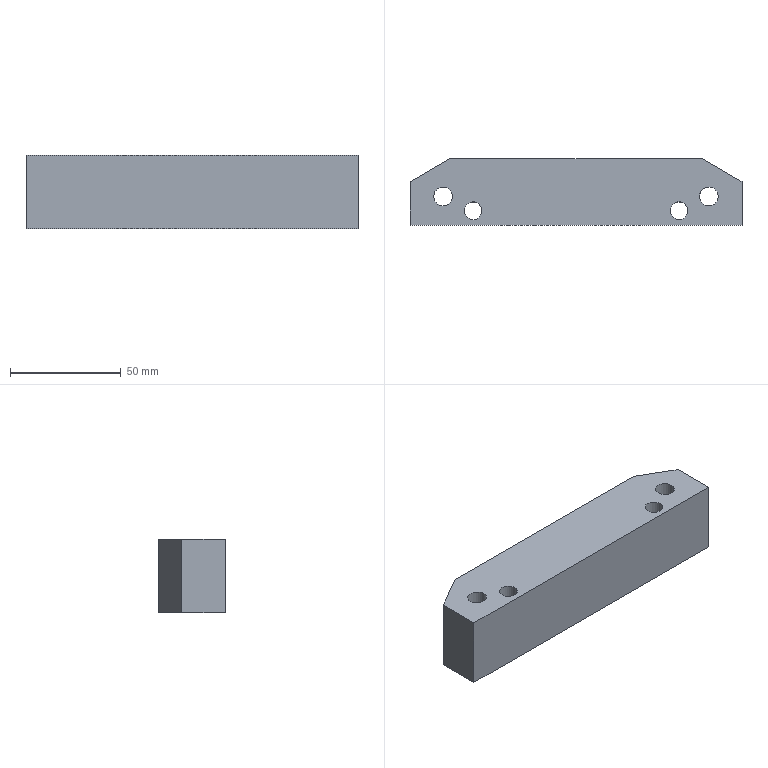Part | CATIA | 1 solid | 16 faces | box 150 x 30 x 33 mm | volume 135264 mm3 | plane 8 | cylinder 8 | commonest cylinder face diameters 8 x4 8.5 x4
STEP:
#1=CARTESIAN_POINT('',(75.,-30.,38.));
#2=VERTEX_POINT('',#1);
#3=CARTESIAN_POINT('',(75.,-30.,5.));
#4=VERTEX_POINT('',#3);
#5=CARTESIAN_POINT('',(75.,-30.,21.5));
#6=DIRECTION('',(0.,0.,-1.));
#7=VECTOR('',#6,1.);
#8=LINE('',#5,#7);
#9=EDGE_CURVE('',#2,#4,#8,.T.);
#10=ORIENTED_EDGE('',*,*,#9,.F.);
#11=CARTESIAN_POINT('',(-75.,-30.,38.));
#12=VERTEX_POINT('',#11);
#13=CARTESIAN_POINT('',(0.,-30.,38.));
#14=DIRECTION('',(-1.,0.,0.));
#15=VECTOR('',#14,1.);
#16=LINE('',#13,#15);
#17=EDGE_CURVE('',#2,#12,#16,.T.);
#18=ORIENTED_EDGE('',*,*,#17,.T.);
#19=CARTESIAN_POINT('',(-75.,-30.,5.));
#20=VERTEX_POINT('',#19);
#21=CARTESIAN_POINT('',(-75.,-30.,21.5));
#22=DIRECTION('',(0.,0.,-1.));
#23=VECTOR('',#22,1.);
#24=LINE('',#21,#23);
#25=EDGE_CURVE('',#12,#20,#24,.T.);
#26=ORIENTED_EDGE('',*,*,#25,.T.);
#27=CARTESIAN_POINT('',(0.,-30.,5.));
#28=DIRECTION('',(-1.,0.,0.));
#29=VECTOR('',#28,1.);
#30=LINE('',#27,#29);
#31=EDGE_CURVE('',#4,#20,#30,.T.);
#32=ORIENTED_EDGE('',*,*,#31,.F.);
#33=EDGE_LOOP('',(#10,#18,#26,#32));
#34=FACE_OUTER_BOUND('',#33,.T.);
#35=CARTESIAN_POINT('',(75.,-30.,38.));
#36=DIRECTION('',(0.,-1.,0.));
#37=DIRECTION('',(-1.,0.,0.));
#38=AXIS2_PLACEMENT_3D('',#35,#36,#37);
#39=PLANE('',#38);
#40=ADVANCED_FACE('',(#34),#39,.T.);
#41=CARTESIAN_POINT('',(-75.,-10.392,38.));
#42=VERTEX_POINT('',#41);
#43=CARTESIAN_POINT('',(-75.,-10.392,5.));
#44=VERTEX_POINT('',#43);
#45=CARTESIAN_POINT('',(-75.,-10.392,21.5));
#46=DIRECTION('',(0.,0.,-1.));
#47=VECTOR('',#46,1.);
#48=LINE('',#45,#47);
#49=EDGE_CURVE('',#42,#44,#48,.T.);
#50=ORIENTED_EDGE('',*,*,#49,.T.);
#51=CARTESIAN_POINT('',(-75.,-20.196,5.));
#52=DIRECTION('',(0.,-1.,0.));
#53=VECTOR('',#52,1.);
#54=LINE('',#51,#53);
#55=EDGE_CURVE('',#20,#44,#54,.F.);
#56=ORIENTED_EDGE('',*,*,#55,.F.);
#57=ORIENTED_EDGE('',*,*,#25,.F.);
#58=CARTESIAN_POINT('',(-75.,-20.196,38.));
#59=DIRECTION('',(0.,-1.,0.));
#60=VECTOR('',#59,1.);
#61=LINE('',#58,#60);
#62=EDGE_CURVE('',#12,#42,#61,.F.);
#63=ORIENTED_EDGE('',*,*,#62,.T.);
#64=EDGE_LOOP('',(#50,#56,#57,#63));
#65=FACE_OUTER_BOUND('',#64,.T.);
#66=CARTESIAN_POINT('',(-75.,0.,38.));
#67=DIRECTION('',(1.,0.,0.));
#68=DIRECTION('',(0.,-1.,0.));
#69=AXIS2_PLACEMENT_3D('',#66,#67,#68);
#70=PLANE('',#69);
#71=ADVANCED_FACE('',(#65),#70,.F.);
#72=CARTESIAN_POINT('',(-57.,0.,5.));
#73=VERTEX_POINT('',#72);
#74=CARTESIAN_POINT('',(-66.,-5.196,5.));
#75=DIRECTION('',(-0.866,-0.5,0.));
#76=VECTOR('',#75,1.);
#77=LINE('',#74,#76);
#78=EDGE_CURVE('',#73,#44,#77,.T.);
#79=ORIENTED_EDGE('',*,*,#78,.T.);
#80=ORIENTED_EDGE('',*,*,#49,.F.);
#81=CARTESIAN_POINT('',(-57.,0.,38.));
#82=VERTEX_POINT('',#81);
#83=CARTESIAN_POINT('',(-66.,-5.196,38.));
#84=DIRECTION('',(-0.866,-0.5,0.));
#85=VECTOR('',#84,1.);
#86=LINE('',#83,#85);
#87=EDGE_CURVE('',#42,#82,#86,.F.);
#88=ORIENTED_EDGE('',*,*,#87,.T.);
#89=CARTESIAN_POINT('',(-57.,0.,21.5));
#90=DIRECTION('',(0.,0.,-1.));
#91=VECTOR('',#90,1.);
#92=LINE('',#89,#91);
#93=EDGE_CURVE('',#82,#73,#92,.T.);
#94=ORIENTED_EDGE('',*,*,#93,.T.);
#95=EDGE_LOOP('',(#79,#80,#88,#94));
#96=FACE_OUTER_BOUND('',#95,.T.);
#97=CARTESIAN_POINT('',(-57.,0.,44.6));
#98=DIRECTION('',(-0.5,0.866,0.));
#99=DIRECTION('',(0.,0.,-1.));
#100=AXIS2_PLACEMENT_3D('',#97,#98,#99);
#101=PLANE('',#100);
#102=ADVANCED_FACE('',(#96),#101,.T.);
#103=CARTESIAN_POINT('',(75.,-10.392,38.));
#104=VERTEX_POINT('',#103);
#105=CARTESIAN_POINT('',(75.,-10.392,5.));
#106=VERTEX_POINT('',#105);
#107=CARTESIAN_POINT('',(75.,-10.392,21.5));
#108=DIRECTION('',(0.,0.,1.));
#109=VECTOR('',#108,1.);
#110=LINE('',#107,#109);
#111=EDGE_CURVE('',#104,#106,#110,.F.);
#112=ORIENTED_EDGE('',*,*,#111,.F.);
#113=CARTESIAN_POINT('',(75.,-20.196,38.));
#114=DIRECTION('',(0.,1.,0.));
#115=VECTOR('',#114,1.);
#116=LINE('',#113,#115);
#117=EDGE_CURVE('',#104,#2,#116,.F.);
#118=ORIENTED_EDGE('',*,*,#117,.T.);
#119=ORIENTED_EDGE('',*,*,#9,.T.);
#120=CARTESIAN_POINT('',(75.,-20.196,5.));
#121=DIRECTION('',(0.,1.,0.));
#122=VECTOR('',#121,1.);
#123=LINE('',#120,#122);
#124=EDGE_CURVE('',#106,#4,#123,.F.);
#125=ORIENTED_EDGE('',*,*,#124,.F.);
#126=EDGE_LOOP('',(#112,#118,#119,#125));
#127=FACE_OUTER_BOUND('',#126,.T.);
#128=CARTESIAN_POINT('',(75.,-30.,38.));
#129=DIRECTION('',(-1.,0.,0.));
#130=DIRECTION('',(0.,1.,0.));
#131=AXIS2_PLACEMENT_3D('',#128,#129,#130);
#132=PLANE('',#131);
#133=ADVANCED_FACE('',(#127),#132,.F.);
#134=CARTESIAN_POINT('',(57.,0.,5.));
#135=VERTEX_POINT('',#134);
#136=CARTESIAN_POINT('',(0.,0.,5.));
#137=DIRECTION('',(1.,0.,0.));
#138=VECTOR('',#137,1.);
#139=LINE('',#136,#138);
#140=EDGE_CURVE('',#73,#135,#139,.T.);
#141=ORIENTED_EDGE('',*,*,#140,.F.);
#142=ORIENTED_EDGE('',*,*,#93,.F.);
#143=CARTESIAN_POINT('',(57.,0.,38.));
#144=VERTEX_POINT('',#143);
#145=CARTESIAN_POINT('',(0.,0.,38.));
#146=DIRECTION('',(1.,0.,0.));
#147=VECTOR('',#146,1.);
#148=LINE('',#145,#147);
#149=EDGE_CURVE('',#82,#144,#148,.T.);
#150=ORIENTED_EDGE('',*,*,#149,.T.);
#151=CARTESIAN_POINT('',(57.,0.,21.5));
#152=DIRECTION('',(0.,0.,1.));
#153=VECTOR('',#152,1.);
#154=LINE('',#151,#153);
#155=EDGE_CURVE('',#144,#135,#154,.F.);
#156=ORIENTED_EDGE('',*,*,#155,.T.);
#157=EDGE_LOOP('',(#141,#142,#150,#156));
#158=FACE_OUTER_BOUND('',#157,.T.);
#159=CARTESIAN_POINT('',(-75.,0.,38.));
#160=DIRECTION('',(0.,1.,0.));
#161=DIRECTION('',(1.,0.,0.));
#162=AXIS2_PLACEMENT_3D('',#159,#160,#161);
#163=PLANE('',#162);
#164=ADVANCED_FACE('',(#158),#163,.T.);
#165=CARTESIAN_POINT('',(66.,-5.196,5.));
#166=DIRECTION('',(0.866,-0.5,0.));
#167=VECTOR('',#166,1.);
#168=LINE('',#165,#167);
#169=EDGE_CURVE('',#106,#135,#168,.F.);
#170=ORIENTED_EDGE('',*,*,#169,.T.);
#171=ORIENTED_EDGE('',*,*,#155,.F.);
#172=CARTESIAN_POINT('',(66.,-5.196,38.));
#173=DIRECTION('',(0.866,-0.5,0.));
#174=VECTOR('',#173,1.);
#175=LINE('',#172,#174);
#176=EDGE_CURVE('',#144,#104,#175,.T.);
#177=ORIENTED_EDGE('',*,*,#176,.T.);
#178=ORIENTED_EDGE('',*,*,#111,.T.);
#179=EDGE_LOOP('',(#170,#171,#177,#178));
#180=FACE_OUTER_BOUND('',#179,.T.);
#181=CARTESIAN_POINT('',(57.,0.,-1.6));
#182=DIRECTION('',(0.5,0.866,0.));
#183=DIRECTION('',(0.,0.,1.));
#184=AXIS2_PLACEMENT_3D('',#181,#182,#183);
#185=PLANE('',#184);
#186=ADVANCED_FACE('',(#180),#185,.T.);
#187=ORIENTED_EDGE('',*,*,#124,.T.);
#188=ORIENTED_EDGE('',*,*,#31,.T.);
#189=ORIENTED_EDGE('',*,*,#55,.T.);
#190=ORIENTED_EDGE('',*,*,#78,.F.);
#191=ORIENTED_EDGE('',*,*,#140,.T.);
#192=ORIENTED_EDGE('',*,*,#169,.F.);
#193=EDGE_LOOP('',(#187,#188,#189,#190,#191,#192));
#194=FACE_OUTER_BOUND('',#193,.T.);
#195=CARTESIAN_POINT('',(-63.73,-14.962,5.));
#196=VERTEX_POINT('',#195);
#197=CARTESIAN_POINT('',(-56.27,-19.038,5.));
#198=VERTEX_POINT('',#197);
#199=CARTESIAN_POINT('',(-60.,-17.,5.));
#200=DIRECTION('',(0.,0.,-1.));
#201=AXIS2_PLACEMENT_3D('',#199,#200,$);
#202=CIRCLE('',#201,4.25);
#203=EDGE_CURVE('',#196,#198,#202,.T.);
#204=ORIENTED_EDGE('',*,*,#203,.F.);
#205=CARTESIAN_POINT('',(-60.,-17.,5.));
#206=DIRECTION('',(0.,0.,-1.));
#207=AXIS2_PLACEMENT_3D('',#205,#206,$);
#208=CIRCLE('',#207,4.25);
#209=EDGE_CURVE('',#198,#196,#208,.T.);
#210=ORIENTED_EDGE('',*,*,#209,.F.);
#211=EDGE_LOOP('',(#204,#210));
#212=FACE_BOUND('',#211,.T.);
#213=CARTESIAN_POINT('',(56.27,-14.962,5.));
#214=VERTEX_POINT('',#213);
#215=CARTESIAN_POINT('',(63.73,-19.038,5.));
#216=VERTEX_POINT('',#215);
#217=CARTESIAN_POINT('',(60.,-17.,5.));
#218=DIRECTION('',(0.,0.,-1.));
#219=AXIS2_PLACEMENT_3D('',#217,#218,$);
#220=CIRCLE('',#219,4.25);
#221=EDGE_CURVE('',#214,#216,#220,.T.);
#222=ORIENTED_EDGE('',*,*,#221,.F.);
#223=CARTESIAN_POINT('',(60.,-17.,5.));
#224=DIRECTION('',(0.,0.,-1.));
#225=AXIS2_PLACEMENT_3D('',#223,#224,$);
#226=CIRCLE('',#225,4.25);
#227=EDGE_CURVE('',#216,#214,#226,.T.);
#228=ORIENTED_EDGE('',*,*,#227,.F.);
#229=EDGE_LOOP('',(#222,#228));
#230=FACE_BOUND('',#229,.T.);
#231=CARTESIAN_POINT('',(-50.01,-21.582,5.));
#232=VERTEX_POINT('',#231);
#233=CARTESIAN_POINT('',(-42.99,-25.418,5.));
#234=VERTEX_POINT('',#233);
#235=CARTESIAN_POINT('',(-46.5,-23.5,5.));
#236=DIRECTION('',(0.,0.,-1.));
#237=AXIS2_PLACEMENT_3D('',#235,#236,$);
#238=CIRCLE('',#237,4.);
#239=EDGE_CURVE('',#232,#234,#238,.T.);
#240=ORIENTED_EDGE('',*,*,#239,.F.);
#241=CARTESIAN_POINT('',(-46.5,-23.5,5.));
#242=DIRECTION('',(0.,0.,-1.));
#243=AXIS2_PLACEMENT_3D('',#241,#242,$);
#244=CIRCLE('',#243,4.);
#245=EDGE_CURVE('',#234,#232,#244,.T.);
#246=ORIENTED_EDGE('',*,*,#245,.F.);
#247=EDGE_LOOP('',(#240,#246));
#248=FACE_BOUND('',#247,.T.);
#249=CARTESIAN_POINT('',(42.99,-21.582,5.));
#250=VERTEX_POINT('',#249);
#251=CARTESIAN_POINT('',(50.01,-25.418,5.));
#252=VERTEX_POINT('',#251);
#253=CARTESIAN_POINT('',(46.5,-23.5,5.));
#254=DIRECTION('',(0.,0.,-1.));
#255=AXIS2_PLACEMENT_3D('',#253,#254,$);
#256=CIRCLE('',#255,4.);
#257=EDGE_CURVE('',#250,#252,#256,.T.);
#258=ORIENTED_EDGE('',*,*,#257,.F.);
#259=CARTESIAN_POINT('',(46.5,-23.5,5.));
#260=DIRECTION('',(0.,0.,-1.));
#261=AXIS2_PLACEMENT_3D('',#259,#260,$);
#262=CIRCLE('',#261,4.);
#263=EDGE_CURVE('',#252,#250,#262,.T.);
#264=ORIENTED_EDGE('',*,*,#263,.F.);
#265=EDGE_LOOP('',(#258,#264));
#266=FACE_BOUND('',#265,.T.);
#267=CARTESIAN_POINT('',(0.,0.,5.));
#268=DIRECTION('',(0.,0.,-1.));
#269=DIRECTION('',(1.,0.,0.));
#270=AXIS2_PLACEMENT_3D('',#267,#268,#269);
#271=PLANE('',#270);
#272=ADVANCED_FACE('',(#194,#212,#230,#248,#266),#271,.T.);
#273=ORIENTED_EDGE('',*,*,#176,.F.);
#274=ORIENTED_EDGE('',*,*,#149,.F.);
#275=ORIENTED_EDGE('',*,*,#87,.F.);
#276=ORIENTED_EDGE('',*,*,#62,.F.);
#277=ORIENTED_EDGE('',*,*,#17,.F.);
#278=ORIENTED_EDGE('',*,*,#117,.F.);
#279=EDGE_LOOP('',(#273,#274,#275,#276,#277,#278));
#280=FACE_OUTER_BOUND('',#279,.T.);
#281=CARTESIAN_POINT('',(-63.73,-14.962,38.));
#282=VERTEX_POINT('',#281);
#283=CARTESIAN_POINT('',(-56.27,-19.038,38.));
#284=VERTEX_POINT('',#283);
#285=CARTESIAN_POINT('',(-60.,-17.,38.));
#286=DIRECTION('',(0.,0.,-1.));
#287=AXIS2_PLACEMENT_3D('',#285,#286,$);
#288=CIRCLE('',#287,4.25);
#289=EDGE_CURVE('',#282,#284,#288,.T.);
#290=ORIENTED_EDGE('',*,*,#289,.T.);
#291=CARTESIAN_POINT('',(-60.,-17.,38.));
#292=DIRECTION('',(0.,0.,-1.));
#293=AXIS2_PLACEMENT_3D('',#291,#292,$);
#294=CIRCLE('',#293,4.25);
#295=EDGE_CURVE('',#284,#282,#294,.T.);
#296=ORIENTED_EDGE('',*,*,#295,.T.);
#297=EDGE_LOOP('',(#290,#296));
#298=FACE_BOUND('',#297,.T.);
#299=CARTESIAN_POINT('',(56.27,-14.962,38.));
#300=VERTEX_POINT('',#299);
#301=CARTESIAN_POINT('',(63.73,-19.038,38.));
#302=VERTEX_POINT('',#301);
#303=CARTESIAN_POINT('',(60.,-17.,38.));
#304=DIRECTION('',(0.,0.,-1.));
#305=AXIS2_PLACEMENT_3D('',#303,#304,$);
#306=CIRCLE('',#305,4.25);
#307=EDGE_CURVE('',#300,#302,#306,.T.);
#308=ORIENTED_EDGE('',*,*,#307,.T.);
#309=CARTESIAN_POINT('',(60.,-17.,38.));
#310=DIRECTION('',(0.,0.,-1.));
#311=AXIS2_PLACEMENT_3D('',#309,#310,$);
#312=CIRCLE('',#311,4.25);
#313=EDGE_CURVE('',#302,#300,#312,.T.);
#314=ORIENTED_EDGE('',*,*,#313,.T.);
#315=EDGE_LOOP('',(#308,#314));
#316=FACE_BOUND('',#315,.T.);
#317=CARTESIAN_POINT('',(-50.01,-21.582,38.));
#318=VERTEX_POINT('',#317);
#319=CARTESIAN_POINT('',(-42.99,-25.418,38.));
#320=VERTEX_POINT('',#319);
#321=CARTESIAN_POINT('',(-46.5,-23.5,38.));
#322=DIRECTION('',(0.,0.,-1.));
#323=AXIS2_PLACEMENT_3D('',#321,#322,$);
#324=CIRCLE('',#323,4.);
#325=EDGE_CURVE('',#318,#320,#324,.T.);
#326=ORIENTED_EDGE('',*,*,#325,.T.);
#327=CARTESIAN_POINT('',(-46.5,-23.5,38.));
#328=DIRECTION('',(0.,0.,-1.));
#329=AXIS2_PLACEMENT_3D('',#327,#328,$);
#330=CIRCLE('',#329,4.);
#331=EDGE_CURVE('',#320,#318,#330,.T.);
#332=ORIENTED_EDGE('',*,*,#331,.T.);
#333=EDGE_LOOP('',(#326,#332));
#334=FACE_BOUND('',#333,.T.);
#335=CARTESIAN_POINT('',(42.99,-21.582,38.));
#336=VERTEX_POINT('',#335);
#337=CARTESIAN_POINT('',(50.01,-25.418,38.));
#338=VERTEX_POINT('',#337);
#339=CARTESIAN_POINT('',(46.5,-23.5,38.));
#340=DIRECTION('',(0.,0.,-1.));
#341=AXIS2_PLACEMENT_3D('',#339,#340,$);
#342=CIRCLE('',#341,4.);
#343=EDGE_CURVE('',#336,#338,#342,.T.);
#344=ORIENTED_EDGE('',*,*,#343,.T.);
#345=CARTESIAN_POINT('',(46.5,-23.5,38.));
#346=DIRECTION('',(0.,0.,-1.));
#347=AXIS2_PLACEMENT_3D('',#345,#346,$);
#348=CIRCLE('',#347,4.);
#349=EDGE_CURVE('',#338,#336,#348,.T.);
#350=ORIENTED_EDGE('',*,*,#349,.T.);
#351=EDGE_LOOP('',(#344,#350));
#352=FACE_BOUND('',#351,.T.);
#353=CARTESIAN_POINT('',(0.,0.,38.));
#354=DIRECTION('',(0.,0.,-1.));
#355=DIRECTION('',(1.,0.,0.));
#356=AXIS2_PLACEMENT_3D('',#353,#354,#355);
#357=PLANE('',#356);
#358=ADVANCED_FACE('',(#280,#298,#316,#334,#352),#357,.F.);
#359=ORIENTED_EDGE('',*,*,#331,.F.);
#360=CARTESIAN_POINT('',(-42.99,-25.418,21.5));
#361=DIRECTION('',(0.,0.,-1.));
#362=VECTOR('',#361,1.);
#363=LINE('',#360,#362);
#364=EDGE_CURVE('',#234,#320,#363,.F.);
#365=ORIENTED_EDGE('',*,*,#364,.F.);
#366=ORIENTED_EDGE('',*,*,#245,.T.);
#367=CARTESIAN_POINT('',(-50.01,-21.582,21.5));
#368=DIRECTION('',(0.,0.,-1.));
#369=VECTOR('',#368,1.);
#370=LINE('',#367,#369);
#371=EDGE_CURVE('',#232,#318,#370,.F.);
#372=ORIENTED_EDGE('',*,*,#371,.T.);
#373=EDGE_LOOP('',(#359,#365,#366,#372));
#374=FACE_OUTER_BOUND('',#373,.T.);
#375=CARTESIAN_POINT('',(-46.5,-23.5,37.9));
#376=DIRECTION('',(0.,0.,-1.));
#377=DIRECTION('',(0.8776,-0.4794,0.));
#378=AXIS2_PLACEMENT_3D('',#375,#376,#377);
#379=CYLINDRICAL_SURFACE('',#378,4.);
#380=ADVANCED_FACE('',(#374),#379,.F.);
#381=ORIENTED_EDGE('',*,*,#325,.F.);
#382=ORIENTED_EDGE('',*,*,#371,.F.);
#383=ORIENTED_EDGE('',*,*,#239,.T.);
#384=ORIENTED_EDGE('',*,*,#364,.T.);
#385=EDGE_LOOP('',(#381,#382,#383,#384));
#386=FACE_OUTER_BOUND('',#385,.T.);
#387=ADVANCED_FACE('',(#386),#379,.F.);
#388=ORIENTED_EDGE('',*,*,#313,.F.);
#389=CARTESIAN_POINT('',(63.73,-19.038,21.5));
#390=DIRECTION('',(0.,0.,-1.));
#391=VECTOR('',#390,1.);
#392=LINE('',#389,#391);
#393=EDGE_CURVE('',#216,#302,#392,.F.);
#394=ORIENTED_EDGE('',*,*,#393,.F.);
#395=ORIENTED_EDGE('',*,*,#227,.T.);
#396=CARTESIAN_POINT('',(56.27,-14.962,21.5));
#397=DIRECTION('',(0.,0.,-1.));
#398=VECTOR('',#397,1.);
#399=LINE('',#396,#398);
#400=EDGE_CURVE('',#214,#300,#399,.F.);
#401=ORIENTED_EDGE('',*,*,#400,.T.);
#402=EDGE_LOOP('',(#388,#394,#395,#401));
#403=FACE_OUTER_BOUND('',#402,.T.);
#404=CARTESIAN_POINT('',(60.,-17.,37.9));
#405=DIRECTION('',(0.,0.,-1.));
#406=DIRECTION('',(0.8776,-0.4794,0.));
#407=AXIS2_PLACEMENT_3D('',#404,#405,#406);
#408=CYLINDRICAL_SURFACE('',#407,4.25);
#409=ADVANCED_FACE('',(#403),#408,.F.);
#410=ORIENTED_EDGE('',*,*,#307,.F.);
#411=ORIENTED_EDGE('',*,*,#400,.F.);
#412=ORIENTED_EDGE('',*,*,#221,.T.);
#413=ORIENTED_EDGE('',*,*,#393,.T.);
#414=EDGE_LOOP('',(#410,#411,#412,#413));
#415=FACE_OUTER_BOUND('',#414,.T.);
#416=ADVANCED_FACE('',(#415),#408,.F.);
#417=ORIENTED_EDGE('',*,*,#349,.F.);
#418=CARTESIAN_POINT('',(50.01,-25.418,21.5));
#419=DIRECTION('',(0.,0.,-1.));
#420=VECTOR('',#419,1.);
#421=LINE('',#418,#420);
#422=EDGE_CURVE('',#252,#338,#421,.F.);
#423=ORIENTED_EDGE('',*,*,#422,.F.);
#424=ORIENTED_EDGE('',*,*,#263,.T.);
#425=CARTESIAN_POINT('',(42.99,-21.582,21.5));
#426=DIRECTION('',(0.,0.,-1.));
#427=VECTOR('',#426,1.);
#428=LINE('',#425,#427);
#429=EDGE_CURVE('',#250,#336,#428,.F.);
#430=ORIENTED_EDGE('',*,*,#429,.T.);
#431=EDGE_LOOP('',(#417,#423,#424,#430));
#432=FACE_OUTER_BOUND('',#431,.T.);
#433=CARTESIAN_POINT('',(46.5,-23.5,37.9));
#434=DIRECTION('',(0.,0.,-1.));
#435=DIRECTION('',(0.8776,-0.4794,0.));
#436=AXIS2_PLACEMENT_3D('',#433,#434,#435);
#437=CYLINDRICAL_SURFACE('',#436,4.);
#438=ADVANCED_FACE('',(#432),#437,.F.);
#439=ORIENTED_EDGE('',*,*,#343,.F.);
#440=ORIENTED_EDGE('',*,*,#429,.F.);
#441=ORIENTED_EDGE('',*,*,#257,.T.);
#442=ORIENTED_EDGE('',*,*,#422,.T.);
#443=EDGE_LOOP('',(#439,#440,#441,#442));
#444=FACE_OUTER_BOUND('',#443,.T.);
#445=ADVANCED_FACE('',(#444),#437,.F.);
#446=ORIENTED_EDGE('',*,*,#295,.F.);
#447=CARTESIAN_POINT('',(-56.27,-19.038,21.5));
#448=DIRECTION('',(0.,0.,-1.));
#449=VECTOR('',#448,1.);
#450=LINE('',#447,#449);
#451=EDGE_CURVE('',#198,#284,#450,.F.);
#452=ORIENTED_EDGE('',*,*,#451,.F.);
#453=ORIENTED_EDGE('',*,*,#209,.T.);
#454=CARTESIAN_POINT('',(-63.73,-14.962,21.5));
#455=DIRECTION('',(0.,0.,-1.));
#456=VECTOR('',#455,1.);
#457=LINE('',#454,#456);
#458=EDGE_CURVE('',#196,#282,#457,.F.);
#459=ORIENTED_EDGE('',*,*,#458,.T.);
#460=EDGE_LOOP('',(#446,#452,#453,#459));
#461=FACE_OUTER_BOUND('',#460,.T.);
#462=CARTESIAN_POINT('',(-60.,-17.,37.9));
#463=DIRECTION('',(0.,0.,-1.));
#464=DIRECTION('',(0.8776,-0.4794,0.));
#465=AXIS2_PLACEMENT_3D('',#462,#463,#464);
#466=CYLINDRICAL_SURFACE('',#465,4.25);
#467=ADVANCED_FACE('',(#461),#466,.F.);
#468=ORIENTED_EDGE('',*,*,#289,.F.);
#469=ORIENTED_EDGE('',*,*,#458,.F.);
#470=ORIENTED_EDGE('',*,*,#203,.T.);
#471=ORIENTED_EDGE('',*,*,#451,.T.);
#472=EDGE_LOOP('',(#468,#469,#470,#471));
#473=FACE_OUTER_BOUND('',#472,.T.);
#474=ADVANCED_FACE('',(#473),#466,.F.);
#475=CLOSED_SHELL('',(#40,#71,#102,#133,#164,#186,#272,#358,#380,#387,#409,#416,#438,#445,#467,#474));
#476=MANIFOLD_SOLID_BREP('',#475);
#477=(LENGTH_UNIT()NAMED_UNIT(*)SI_UNIT(.MILLI.,.METRE.));
#478=UNCERTAINTY_MEASURE_WITH_UNIT(LENGTH_MEASURE(0.005),#477,'','');
#479=(NAMED_UNIT(*)PLANE_ANGLE_UNIT()SI_UNIT($,.RADIAN.));
#480=(NAMED_UNIT(*)SI_UNIT($,.STERADIAN.)SOLID_ANGLE_UNIT());
#481=(GEOMETRIC_REPRESENTATION_CONTEXT(3)GLOBAL_UNCERTAINTY_ASSIGNED_CONTEXT((#478))GLOBAL_UNIT_ASSIGNED_CONTEXT((#477,#479,#480))REPRESENTATION_CONTEXT('',''));
#482=ADVANCED_BREP_SHAPE_REPRESENTATION('',(#476),#481);